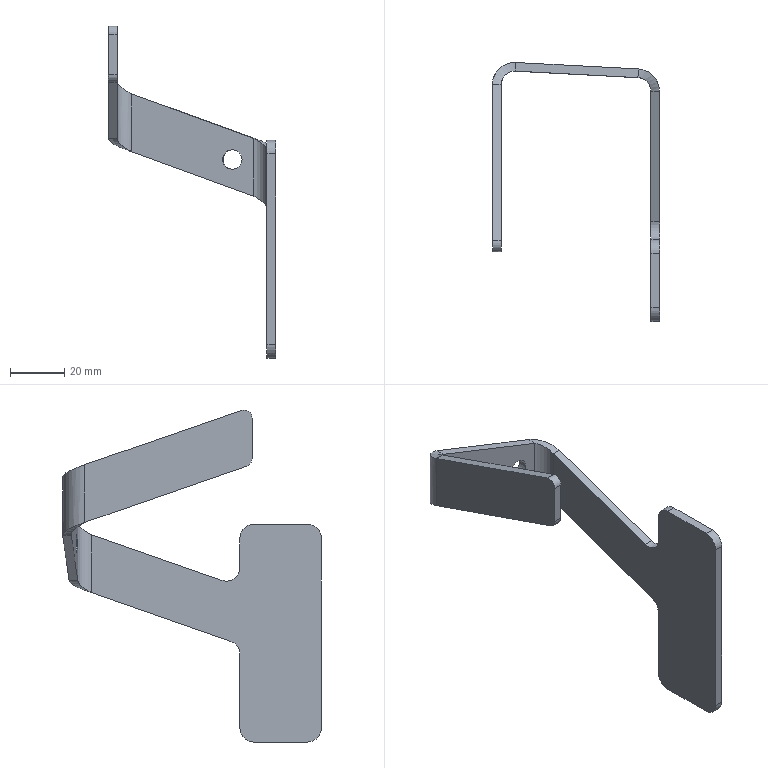Part | SolidWorks | features EdgeFlange 2, Fillet 2, ICE 2, FlatPattern 1, RefAxis 1, SMBaseFlange 1, SheetMetal 1 | 1 solid | 36 faces | box 61.639 x 95.405 x 122.483 mm | volume 19991 mm3 | plane 18 | cylinder 14 | spline 4 | commonest cylinder face diameters 10 x8 6 x2 7.2 x2 16.4 x2
STEP:
#1=CARTESIAN_POINT('',(3.429,-3.382,0.));
#2=VERTEX_POINT('',#1);
#3=CARTESIAN_POINT('',(-3.761,-3.009,0.));
#4=VERTEX_POINT('',#3);
#5=CARTESIAN_POINT('',(-0.166,-3.196,0.));
#6=DIRECTION('',(0.05188,0.9987,0.));
#7=DIRECTION('',(-0.9987,0.05188,0.));
#8=AXIS2_PLACEMENT_3D('',#5,#6,#7);
#9=CIRCLE('',#8,3.6);
#10=EDGE_CURVE('',#2,#4,#9,.T.);
#11=ORIENTED_EDGE('',*,*,#10,.F.);
#12=CARTESIAN_POINT('',(3.595,-0.1868,0.));
#13=VERTEX_POINT('',#12);
#14=CARTESIAN_POINT('',(3.076,-10.173,0.));
#15=DIRECTION('',(0.05188,0.9987,0.));
#16=VECTOR('',#15,1000.);
#17=LINE('',#14,#16);
#18=EDGE_CURVE('',#2,#13,#17,.T.);
#19=ORIENTED_EDGE('',*,*,#18,.T.);
#20=CARTESIAN_POINT('',(-3.595,0.1868,0.));
#21=VERTEX_POINT('',#20);
#22=CARTESIAN_POINT('',(0.,0.,0.));
#23=DIRECTION('',(0.05188,0.9987,0.));
#24=DIRECTION('',(-0.9987,0.05188,0.));
#25=AXIS2_PLACEMENT_3D('',#22,#23,#24);
#26=CIRCLE('',#25,3.6);
#27=EDGE_CURVE('',#13,#21,#26,.T.);
#28=ORIENTED_EDGE('',*,*,#27,.T.);
#29=CARTESIAN_POINT('',(-4.114,-9.8,0.));
#30=DIRECTION('',(0.05188,0.9987,0.));
#31=VECTOR('',#30,1000.);
#32=LINE('',#29,#31);
#33=EDGE_CURVE('',#4,#21,#32,.T.);
#34=ORIENTED_EDGE('',*,*,#33,.F.);
#35=EDGE_LOOP('',(#11,#19,#28,#34));
#36=FACE_OUTER_BOUND('',#35,.T.);
#37=CARTESIAN_POINT('',(-0.5188,-9.987,0.));
#38=DIRECTION('',(0.05188,0.9987,0.));
#39=DIRECTION('',(-0.9987,0.05188,0.));
#40=AXIS2_PLACEMENT_3D('',#37,#38,#39);
#41=CYLINDRICAL_SURFACE('',#40,3.6);
#42=ADVANCED_FACE('',(#36),#41,.F.);
#43=CARTESIAN_POINT('',(-0.166,-3.196,0.));
#44=DIRECTION('',(0.05188,0.9987,0.));
#45=DIRECTION('',(-0.9987,0.05188,0.));
#46=AXIS2_PLACEMENT_3D('',#43,#44,#45);
#47=CIRCLE('',#46,3.6);
#48=EDGE_CURVE('',#4,#2,#47,.T.);
#49=ORIENTED_EDGE('',*,*,#48,.T.);
#50=ORIENTED_EDGE('',*,*,#10,.T.);
#51=EDGE_LOOP('',(#49,#50));
#52=FACE_BOUND('',#51,.T.);
#53=CARTESIAN_POINT('',(7.795,-3.609,7.804));
#54=VERTEX_POINT('',#53);
#55=CARTESIAN_POINT('',(7.795,-3.609,-13.54));
#56=VERTEX_POINT('',#55);
#57=CARTESIAN_POINT('',(7.795,-3.609,7.804));
#58=DIRECTION('',(0.,0.,-1.));
#59=VECTOR('',#58,1000.);
#60=LINE('',#57,#59);
#61=EDGE_CURVE('',#54,#56,#60,.T.);
#62=ORIENTED_EDGE('',*,*,#61,.F.);
#63=CARTESIAN_POINT('',(-37.404,-1.261,24.256));
#64=VERTEX_POINT('',#63);
#65=CARTESIAN_POINT('',(-53.293,-0.4358,30.039));
#66=DIRECTION('',(-0.9386,0.04876,0.3416));
#67=VECTOR('',#66,1000.);
#68=LINE('',#65,#67);
#69=EDGE_CURVE('',#54,#64,#68,.T.);
#70=ORIENTED_EDGE('',*,*,#69,.T.);
#71=CARTESIAN_POINT('',(-37.404,-1.261,2.912));
#72=VERTEX_POINT('',#71);
#73=CARTESIAN_POINT('',(-37.404,-1.261,2.912));
#74=DIRECTION('',(0.,0.,1.));
#75=VECTOR('',#74,1000.);
#76=LINE('',#73,#75);
#77=EDGE_CURVE('',#72,#64,#76,.T.);
#78=ORIENTED_EDGE('',*,*,#77,.F.);
#79=CARTESIAN_POINT('',(-60.137,-0.08033,11.186));
#80=DIRECTION('',(0.9386,-0.04876,-0.3416));
#81=VECTOR('',#80,1000.);
#82=LINE('',#79,#81);
#83=EDGE_CURVE('',#72,#56,#82,.T.);
#84=ORIENTED_EDGE('',*,*,#83,.T.);
#85=EDGE_LOOP('',(#62,#70,#78,#84));
#86=FACE_OUTER_BOUND('',#85,.T.);
#87=CARTESIAN_POINT('',(-45.866,-0.8217,50.5));
#88=DIRECTION('',(0.05188,0.9987,0.));
#89=DIRECTION('',(-0.9987,0.05188,0.));
#90=AXIS2_PLACEMENT_3D('',#87,#88,#89);
#91=PLANE('',#90);
#92=ADVANCED_FACE('',(#52,#86),#91,.F.);
#93=CARTESIAN_POINT('',(0.,0.,0.));
#94=DIRECTION('',(0.05188,0.9987,0.));
#95=DIRECTION('',(-0.9987,0.05188,0.));
#96=AXIS2_PLACEMENT_3D('',#93,#94,#95);
#97=CIRCLE('',#96,3.6);
#98=EDGE_CURVE('',#21,#13,#97,.T.);
#99=ORIENTED_EDGE('',*,*,#98,.F.);
#100=ORIENTED_EDGE('',*,*,#27,.F.);
#101=EDGE_LOOP('',(#99,#100));
#102=FACE_BOUND('',#101,.T.);
#103=CARTESIAN_POINT('',(7.961,-0.4136,7.804));
#104=VERTEX_POINT('',#103);
#105=CARTESIAN_POINT('',(-37.238,1.934,24.256));
#106=VERTEX_POINT('',#105);
#107=CARTESIAN_POINT('',(-53.127,2.76,30.039));
#108=DIRECTION('',(-0.9386,0.04876,0.3416));
#109=VECTOR('',#108,1000.);
#110=LINE('',#107,#109);
#111=EDGE_CURVE('',#104,#106,#110,.T.);
#112=ORIENTED_EDGE('',*,*,#111,.F.);
#113=CARTESIAN_POINT('',(7.961,-0.4136,-13.54));
#114=VERTEX_POINT('',#113);
#115=CARTESIAN_POINT('',(7.961,-0.4136,7.804));
#116=DIRECTION('',(0.,0.,-1.));
#117=VECTOR('',#116,1000.);
#118=LINE('',#115,#117);
#119=EDGE_CURVE('',#104,#114,#118,.T.);
#120=ORIENTED_EDGE('',*,*,#119,.T.);
#121=CARTESIAN_POINT('',(-37.238,1.934,2.912));
#122=VERTEX_POINT('',#121);
#123=CARTESIAN_POINT('',(-59.971,3.115,11.186));
#124=DIRECTION('',(0.9386,-0.04876,-0.3416));
#125=VECTOR('',#124,1000.);
#126=LINE('',#123,#125);
#127=EDGE_CURVE('',#122,#114,#126,.T.);
#128=ORIENTED_EDGE('',*,*,#127,.F.);
#129=CARTESIAN_POINT('',(-37.238,1.934,2.912));
#130=DIRECTION('',(0.,0.,1.));
#131=VECTOR('',#130,1000.);
#132=LINE('',#129,#131);
#133=EDGE_CURVE('',#122,#106,#132,.T.);
#134=ORIENTED_EDGE('',*,*,#133,.T.);
#135=EDGE_LOOP('',(#112,#120,#128,#134));
#136=FACE_OUTER_BOUND('',#135,.T.);
#137=CARTESIAN_POINT('',(-45.7,2.374,50.5));
#138=DIRECTION('',(0.05188,0.9987,0.));
#139=DIRECTION('',(-0.9987,0.05188,0.));
#140=AXIS2_PLACEMENT_3D('',#137,#138,#139);
#141=PLANE('',#140);
#142=ADVANCED_FACE('',(#102,#136),#141,.T.);
#143=CARTESIAN_POINT('',(7.795,-3.609,7.804));
#144=DIRECTION('',(0.05188,0.9987,0.));
#145=VECTOR('',#144,1000.);
#146=LINE('',#143,#145);
#147=EDGE_CURVE('',#54,#104,#146,.T.);
#148=ORIENTED_EDGE('',*,*,#147,.T.);
#149=ORIENTED_EDGE('',*,*,#111,.T.);
#150=CARTESIAN_POINT('',(-37.404,-1.261,24.256));
#151=DIRECTION('',(0.05188,0.9987,0.));
#152=VECTOR('',#151,1000.);
#153=LINE('',#150,#152);
#154=EDGE_CURVE('',#64,#106,#153,.T.);
#155=ORIENTED_EDGE('',*,*,#154,.F.);
#156=ORIENTED_EDGE('',*,*,#69,.F.);
#157=EDGE_LOOP('',(#148,#149,#155,#156));
#158=FACE_OUTER_BOUND('',#157,.T.);
#159=CARTESIAN_POINT('',(-53.127,2.76,30.039));
#160=DIRECTION('',(0.3412,-0.01772,0.9398));
#161=DIRECTION('',(-0.9386,0.04876,0.3416));
#162=AXIS2_PLACEMENT_3D('',#159,#160,#161);
#163=PLANE('',#162);
#164=ADVANCED_FACE('',(#158),#163,.T.);
#165=CARTESIAN_POINT('',(7.795,-3.609,-13.54));
#166=DIRECTION('',(0.05188,0.9987,0.));
#167=VECTOR('',#166,1000.);
#168=LINE('',#165,#167);
#169=EDGE_CURVE('',#56,#114,#168,.T.);
#170=ORIENTED_EDGE('',*,*,#169,.F.);
#171=ORIENTED_EDGE('',*,*,#83,.F.);
#172=CARTESIAN_POINT('',(-37.404,-1.261,2.912));
#173=DIRECTION('',(0.05188,0.9987,0.));
#174=VECTOR('',#173,1000.);
#175=LINE('',#172,#174);
#176=EDGE_CURVE('',#72,#122,#175,.T.);
#177=ORIENTED_EDGE('',*,*,#176,.T.);
#178=ORIENTED_EDGE('',*,*,#127,.T.);
#179=EDGE_LOOP('',(#170,#171,#177,#178));
#180=FACE_OUTER_BOUND('',#179,.T.);
#181=CARTESIAN_POINT('',(-59.971,3.115,11.186));
#182=DIRECTION('',(-0.3412,0.01772,-0.9398));
#183=DIRECTION('',(0.9386,-0.04876,-0.3416));
#184=AXIS2_PLACEMENT_3D('',#181,#182,#183);
#185=PLANE('',#184);
#186=ADVANCED_FACE('',(#180),#185,.T.);
#187=CARTESIAN_POINT('',(-42.664,-6.257,29.104));
#188=VERTEX_POINT('',#187);
#189=CARTESIAN_POINT('',(-45.864,-6.258,29.104));
#190=VERTEX_POINT('',#189);
#191=CARTESIAN_POINT('',(-45.864,-6.258,29.104));
#192=DIRECTION('',(-1.,-0.0004585,0.));
#193=VECTOR('',#192,1000.);
#194=LINE('',#191,#193);
#195=EDGE_CURVE('',#188,#190,#194,.T.);
#196=ORIENTED_EDGE('',*,*,#195,.F.);
#197=CARTESIAN_POINT('',(-37.404,-1.261,24.256));
#198=CARTESIAN_POINT('',(-37.745,-1.244,24.46));
#199=CARTESIAN_POINT('',(-38.083,-1.261,24.661));
#200=CARTESIAN_POINT('',(-38.748,-1.362,25.062));
#201=CARTESIAN_POINT('',(-39.077,-1.446,25.264));
#202=CARTESIAN_POINT('',(-39.716,-1.682,25.671));
#203=CARTESIAN_POINT('',(-40.019,-1.831,25.872));
#204=CARTESIAN_POINT('',(-40.59,-2.187,26.274));
#205=CARTESIAN_POINT('',(-40.86,-2.395,26.476));
#206=CARTESIAN_POINT('',(-41.353,-2.863,26.883));
#207=CARTESIAN_POINT('',(-41.573,-3.12,27.083));
#208=CARTESIAN_POINT('',(-41.862,-3.534,27.385));
#209=CARTESIAN_POINT('',(-41.951,-3.677,27.486));
#210=CARTESIAN_POINT('',(-42.116,-3.973,27.688));
#211=CARTESIAN_POINT('',(-42.191,-4.126,27.79));
#212=CARTESIAN_POINT('',(-42.392,-4.595,28.094));
#213=CARTESIAN_POINT('',(-42.493,-4.917,28.295));
#214=CARTESIAN_POINT('',(-42.629,-5.576,28.697));
#215=CARTESIAN_POINT('',(-42.664,-5.916,28.9));
#216=CARTESIAN_POINT('',(-42.664,-6.257,29.104));
#217=B_SPLINE_CURVE_WITH_KNOTS('',3,(#197,#198,#199,#200,#201,#202,#203,#204,#205,#206,#207,#208,#209,#210,#211,#212,#213,#214,#215,#216),.UNSPECIFIED.,.F.,.F.,(4,2,2,2,2,2,2,2,2,4),(0.,0.001176,0.002352,0.003527,0.004703,0.005879,0.006467,0.007055,0.00823,0.009406),.UNSPECIFIED.);
#218=EDGE_CURVE('',#64,#188,#217,.T.);
#219=ORIENTED_EDGE('',*,*,#218,.F.);
#220=ORIENTED_EDGE('',*,*,#154,.T.);
#221=CARTESIAN_POINT('',(-37.238,1.934,24.256));
#222=CARTESIAN_POINT('',(-37.797,1.963,24.46));
#223=CARTESIAN_POINT('',(-38.349,1.935,24.66));
#224=CARTESIAN_POINT('',(-39.167,1.811,24.961));
#225=CARTESIAN_POINT('',(-39.438,1.756,25.062));
#226=CARTESIAN_POINT('',(-39.976,1.618,25.264));
#227=CARTESIAN_POINT('',(-40.244,1.534,25.366));
#228=CARTESIAN_POINT('',(-41.026,1.245,25.67));
#229=CARTESIAN_POINT('',(-41.522,1.002,25.87));
#230=CARTESIAN_POINT('',(-42.461,0.4186,26.273));
#231=CARTESIAN_POINT('',(-42.907,0.07379,26.477));
#232=CARTESIAN_POINT('',(-43.71,-0.6881,26.88));
#233=CARTESIAN_POINT('',(-44.07,-1.106,27.08));
#234=CARTESIAN_POINT('',(-44.546,-1.789,27.383));
#235=CARTESIAN_POINT('',(-44.695,-2.027,27.485));
#236=CARTESIAN_POINT('',(-44.966,-2.513,27.688));
#237=CARTESIAN_POINT('',(-45.088,-2.762,27.789));
#238=CARTESIAN_POINT('',(-45.415,-3.522,28.09));
#239=CARTESIAN_POINT('',(-45.581,-4.049,28.291));
#240=CARTESIAN_POINT('',(-45.807,-5.142,28.697));
#241=CARTESIAN_POINT('',(-45.864,-5.699,28.9));
#242=CARTESIAN_POINT('',(-45.864,-6.258,29.104));
#243=B_SPLINE_CURVE_WITH_KNOTS('',3,(#221,#222,#223,#224,#225,#226,#227,#228,#229,#230,#231,#232,#233,#234,#235,#236,#237,#238,#239,#240,#241,#242),.UNSPECIFIED.,.F.,.F.,(4,2,2,2,2,2,2,2,2,2,4),(0.,0.001761,0.002641,0.003522,0.005283,0.007043,0.008804,0.009685,0.01057,0.01233,0.01409),.UNSPECIFIED.);
#244=EDGE_CURVE('',#106,#190,#243,.T.);
#245=ORIENTED_EDGE('',*,*,#244,.T.);
#246=EDGE_LOOP('',(#196,#219,#220,#245));
#247=FACE_OUTER_BOUND('',#246,.T.);
#248=CARTESIAN_POINT('',(-37.236,1.966,24.256));
#249=CARTESIAN_POINT('',(-38.349,2.024,24.66));
#250=CARTESIAN_POINT('',(-39.472,1.853,25.064));
#251=CARTESIAN_POINT('',(-41.561,1.081,25.872));
#252=CARTESIAN_POINT('',(-42.525,0.481,26.276));
#253=CARTESIAN_POINT('',(-44.14,-1.053,27.084));
#254=CARTESIAN_POINT('',(-44.789,-1.985,27.488));
#255=CARTESIAN_POINT('',(-45.668,-4.032,28.296));
#256=CARTESIAN_POINT('',(-45.896,-5.145,28.7));
#257=CARTESIAN_POINT('',(-45.896,-6.258,29.104));
#258=CARTESIAN_POINT('',(-37.238,1.934,24.256));
#259=CARTESIAN_POINT('',(-38.346,1.992,24.66));
#260=CARTESIAN_POINT('',(-39.465,1.822,25.064));
#261=CARTESIAN_POINT('',(-41.546,1.053,25.872));
#262=CARTESIAN_POINT('',(-42.507,0.4548,26.276));
#263=CARTESIAN_POINT('',(-44.115,-1.073,27.084));
#264=CARTESIAN_POINT('',(-44.762,-2.002,27.488));
#265=CARTESIAN_POINT('',(-45.636,-4.04,28.296));
#266=CARTESIAN_POINT('',(-45.864,-5.149,28.7));
#267=CARTESIAN_POINT('',(-45.864,-6.258,29.104));
#268=CARTESIAN_POINT('',(-37.404,-1.261,24.256));
#269=CARTESIAN_POINT('',(-38.08,-1.226,24.66));
#270=CARTESIAN_POINT('',(-38.762,-1.33,25.064));
#271=CARTESIAN_POINT('',(-40.031,-1.799,25.872));
#272=CARTESIAN_POINT('',(-40.617,-2.163,26.276));
#273=CARTESIAN_POINT('',(-41.597,-3.095,27.084));
#274=CARTESIAN_POINT('',(-41.992,-3.661,27.488));
#275=CARTESIAN_POINT('',(-42.525,-4.904,28.296));
#276=CARTESIAN_POINT('',(-42.664,-5.58,28.7));
#277=CARTESIAN_POINT('',(-42.664,-6.257,29.104));
#278=CARTESIAN_POINT('',(-37.406,-1.294,24.256));
#279=CARTESIAN_POINT('',(-38.077,-1.259,24.66));
#280=CARTESIAN_POINT('',(-38.755,-1.362,25.064));
#281=CARTESIAN_POINT('',(-40.015,-1.828,25.872));
#282=CARTESIAN_POINT('',(-40.597,-2.19,26.276));
#283=CARTESIAN_POINT('',(-41.572,-3.115,27.084));
#284=CARTESIAN_POINT('',(-41.964,-3.678,27.488));
#285=CARTESIAN_POINT('',(-42.494,-4.913,28.296));
#286=CARTESIAN_POINT('',(-42.632,-5.585,28.7));
#287=CARTESIAN_POINT('',(-42.631,-6.257,29.104));
#288=B_SPLINE_SURFACE_WITH_KNOTS('',1,3,((#248,#249,#250,#251,#252,#253,#254,#255,#256,#257),(#258,#259,#260,#261,#262,#263,#264,#265,#266,#267),(#268,#269,#270,#271,#272,#273,#274,#275,#276,#277),(#278,#279,#280,#281,#282,#283,#284,#285,#286,#287)),.UNSPECIFIED.,.F.,.F.,.F.,(2,1,1,2),(4,2,2,2,4),(-0.01,0.,1.,1.01),(0.,0.25,0.5,0.75,1.),.UNSPECIFIED.);
#289=ADVANCED_FACE('',(#247),#288,.F.);
#290=CARTESIAN_POINT('',(-42.664,-6.257,7.82));
#291=VERTEX_POINT('',#290);
#292=CARTESIAN_POINT('',(-42.664,-6.257,7.82));
#293=CARTESIAN_POINT('',(-42.664,-5.915,7.613));
#294=CARTESIAN_POINT('',(-42.629,-5.579,7.41));
#295=CARTESIAN_POINT('',(-42.494,-4.919,7.003));
#296=CARTESIAN_POINT('',(-42.392,-4.595,6.798));
#297=CARTESIAN_POINT('',(-42.123,-3.968,6.386));
#298=CARTESIAN_POINT('',(-41.959,-3.673,6.182));
#299=CARTESIAN_POINT('',(-41.573,-3.12,5.775));
#300=CARTESIAN_POINT('',(-41.352,-2.861,5.57));
#301=CARTESIAN_POINT('',(-40.857,-2.393,5.158));
#302=CARTESIAN_POINT('',(-40.59,-2.186,4.955));
#303=CARTESIAN_POINT('',(-40.161,-1.919,4.649));
#304=CARTESIAN_POINT('',(-40.013,-1.838,4.547));
#305=CARTESIAN_POINT('',(-39.709,-1.689,4.342));
#306=CARTESIAN_POINT('',(-39.551,-1.621,4.239));
#307=CARTESIAN_POINT('',(-38.754,-1.328,3.725));
#308=CARTESIAN_POINT('',(-38.086,-1.226,3.325));
#309=CARTESIAN_POINT('',(-37.404,-1.261,2.912));
#310=B_SPLINE_CURVE_WITH_KNOTS('',3,(#292,#293,#294,#295,#296,#297,#298,#299,#300,#301,#302,#303,#304,#305,#306,#307,#308,#309),.UNSPECIFIED.,.F.,.F.,(4,2,2,2,2,2,2,2,4),(0.,0.001181,0.002361,0.003542,0.004723,0.005903,0.006494,0.007084,0.009446),.UNSPECIFIED.);
#311=EDGE_CURVE('',#291,#72,#310,.T.);
#312=ORIENTED_EDGE('',*,*,#311,.F.);
#313=CARTESIAN_POINT('',(-45.864,-6.258,7.82));
#314=VERTEX_POINT('',#313);
#315=CARTESIAN_POINT('',(-42.664,-6.257,7.82));
#316=DIRECTION('',(-1.,-0.0004585,0.));
#317=VECTOR('',#316,1000.);
#318=LINE('',#315,#317);
#319=EDGE_CURVE('',#291,#314,#318,.T.);
#320=ORIENTED_EDGE('',*,*,#319,.T.);
#321=CARTESIAN_POINT('',(-45.864,-6.258,7.82));
#322=CARTESIAN_POINT('',(-45.864,-5.699,7.614));
#323=CARTESIAN_POINT('',(-45.807,-5.148,7.411));
#324=CARTESIAN_POINT('',(-45.641,-4.338,7.106));
#325=CARTESIAN_POINT('',(-45.572,-4.07,7.004));
#326=CARTESIAN_POINT('',(-45.406,-3.54,6.799));
#327=CARTESIAN_POINT('',(-45.309,-3.277,6.696));
#328=CARTESIAN_POINT('',(-44.98,-2.511,6.388));
#329=CARTESIAN_POINT('',(-44.712,-2.028,6.186));
#330=CARTESIAN_POINT('',(-44.081,-1.12,5.778));
#331=CARTESIAN_POINT('',(-43.714,-0.6921,5.571));
#332=CARTESIAN_POINT('',(-42.912,0.07036,5.163));
#333=CARTESIAN_POINT('',(-42.475,0.4084,4.96));
#334=CARTESIAN_POINT('',(-41.769,0.8489,4.654));
#335=CARTESIAN_POINT('',(-41.524,0.9852,4.55));
#336=CARTESIAN_POINT('',(-41.024,1.23,4.345));
#337=CARTESIAN_POINT('',(-40.77,1.339,4.243));
#338=CARTESIAN_POINT('',(-39.994,1.627,3.938));
#339=CARTESIAN_POINT('',(-39.459,1.766,3.735));
#340=CARTESIAN_POINT('',(-38.356,1.935,3.324));
#341=CARTESIAN_POINT('',(-37.797,1.963,3.118));
#342=CARTESIAN_POINT('',(-37.238,1.934,2.912));
#343=B_SPLINE_CURVE_WITH_KNOTS('',3,(#321,#322,#323,#324,#325,#326,#327,#328,#329,#330,#331,#332,#333,#334,#335,#336,#337,#338,#339,#340,#341,#342),.UNSPECIFIED.,.F.,.F.,(4,2,2,2,2,2,2,2,2,2,4),(0.,0.001763,0.002645,0.003527,0.00529,0.007054,0.008817,0.009699,0.01058,0.01234,0.01411),.UNSPECIFIED.);
#344=EDGE_CURVE('',#314,#122,#343,.T.);
#345=ORIENTED_EDGE('',*,*,#344,.T.);
#346=ORIENTED_EDGE('',*,*,#176,.F.);
#347=EDGE_LOOP('',(#312,#320,#345,#346));
#348=FACE_OUTER_BOUND('',#347,.T.);
#349=CARTESIAN_POINT('',(-45.896,-6.258,7.82));
#350=CARTESIAN_POINT('',(-45.896,-5.145,7.411));
#351=CARTESIAN_POINT('',(-45.668,-4.032,7.002));
#352=CARTESIAN_POINT('',(-44.789,-1.985,6.184));
#353=CARTESIAN_POINT('',(-44.14,-1.053,5.775));
#354=CARTESIAN_POINT('',(-42.525,0.481,4.957));
#355=CARTESIAN_POINT('',(-41.561,1.081,4.548));
#356=CARTESIAN_POINT('',(-39.472,1.853,3.73));
#357=CARTESIAN_POINT('',(-38.349,2.024,3.321));
#358=CARTESIAN_POINT('',(-37.236,1.966,2.912));
#359=CARTESIAN_POINT('',(-45.864,-6.258,7.82));
#360=CARTESIAN_POINT('',(-45.864,-5.149,7.411));
#361=CARTESIAN_POINT('',(-45.636,-4.04,7.002));
#362=CARTESIAN_POINT('',(-44.762,-2.002,6.184));
#363=CARTESIAN_POINT('',(-44.115,-1.073,5.775));
#364=CARTESIAN_POINT('',(-42.507,0.4548,4.957));
#365=CARTESIAN_POINT('',(-41.546,1.053,4.548));
#366=CARTESIAN_POINT('',(-39.465,1.822,3.73));
#367=CARTESIAN_POINT('',(-38.346,1.992,3.321));
#368=CARTESIAN_POINT('',(-37.238,1.934,2.912));
#369=CARTESIAN_POINT('',(-42.664,-6.257,7.82));
#370=CARTESIAN_POINT('',(-42.664,-5.58,7.411));
#371=CARTESIAN_POINT('',(-42.525,-4.904,7.002));
#372=CARTESIAN_POINT('',(-41.992,-3.661,6.184));
#373=CARTESIAN_POINT('',(-41.597,-3.095,5.775));
#374=CARTESIAN_POINT('',(-40.617,-2.163,4.957));
#375=CARTESIAN_POINT('',(-40.031,-1.799,4.548));
#376=CARTESIAN_POINT('',(-38.762,-1.33,3.73));
#377=CARTESIAN_POINT('',(-38.08,-1.226,3.321));
#378=CARTESIAN_POINT('',(-37.404,-1.261,2.912));
#379=CARTESIAN_POINT('',(-42.631,-6.257,7.82));
#380=CARTESIAN_POINT('',(-42.632,-5.585,7.411));
#381=CARTESIAN_POINT('',(-42.494,-4.913,7.002));
#382=CARTESIAN_POINT('',(-41.964,-3.678,6.184));
#383=CARTESIAN_POINT('',(-41.572,-3.115,5.775));
#384=CARTESIAN_POINT('',(-40.597,-2.19,4.957));
#385=CARTESIAN_POINT('',(-40.015,-1.828,4.548));
#386=CARTESIAN_POINT('',(-38.755,-1.362,3.73));
#387=CARTESIAN_POINT('',(-38.077,-1.259,3.321));
#388=CARTESIAN_POINT('',(-37.406,-1.294,2.912));
#389=B_SPLINE_SURFACE_WITH_KNOTS('',1,3,((#349,#350,#351,#352,#353,#354,#355,#356,#357,#358),(#359,#360,#361,#362,#363,#364,#365,#366,#367,#368),(#369,#370,#371,#372,#373,#374,#375,#376,#377,#378),(#379,#380,#381,#382,#383,#384,#385,#386,#387,#388)),.UNSPECIFIED.,.F.,.F.,.F.,(2,1,1,2),(4,2,2,2,4),(-0.01,0.,1.,1.01),(0.,0.25,0.5,0.75,1.),.UNSPECIFIED.);
#390=ADVANCED_FACE('',(#348),#389,.F.);
#391=ORIENTED_EDGE('',*,*,#133,.F.);
#392=ORIENTED_EDGE('',*,*,#344,.F.);
#393=CARTESIAN_POINT('',(-45.864,-6.258,29.104));
#394=DIRECTION('',(0.,0.,1.));
#395=VECTOR('',#394,1000.);
#396=LINE('',#393,#395);
#397=EDGE_CURVE('',#314,#190,#396,.T.);
#398=ORIENTED_EDGE('',*,*,#397,.T.);
#399=ORIENTED_EDGE('',*,*,#244,.F.);
#400=EDGE_LOOP('',(#391,#392,#398,#399));
#401=FACE_OUTER_BOUND('',#400,.T.);
#402=CARTESIAN_POINT('',(-37.664,-6.255,2.912));
#403=DIRECTION('',(0.,0.,-1.));
#404=DIRECTION('',(-1.,-0.0004585,0.));
#405=AXIS2_PLACEMENT_3D('',#402,#403,#404);
#406=CYLINDRICAL_SURFACE('',#405,8.2);
#407=ADVANCED_FACE('',(#401),#406,.T.);
#408=ORIENTED_EDGE('',*,*,#77,.T.);
#409=ORIENTED_EDGE('',*,*,#218,.T.);
#410=CARTESIAN_POINT('',(-42.664,-6.257,29.104));
#411=DIRECTION('',(0.,0.,-1.));
#412=VECTOR('',#411,1000.);
#413=LINE('',#410,#412);
#414=EDGE_CURVE('',#188,#291,#413,.T.);
#415=ORIENTED_EDGE('',*,*,#414,.T.);
#416=ORIENTED_EDGE('',*,*,#311,.T.);
#417=EDGE_LOOP('',(#408,#409,#415,#416));
#418=FACE_OUTER_BOUND('',#417,.T.);
#419=CARTESIAN_POINT('',(-37.664,-6.255,2.912));
#420=DIRECTION('',(0.,0.,-1.));
#421=DIRECTION('',(-1.,-0.0004585,0.));
#422=AXIS2_PLACEMENT_3D('',#419,#420,#421);
#423=CYLINDRICAL_SURFACE('',#422,5.);
#424=ADVANCED_FACE('',(#418),#423,.F.);
#425=CARTESIAN_POINT('',(-42.636,-65.899,28.517));
#426=VERTEX_POINT('',#425);
#427=CARTESIAN_POINT('',(-42.635,-67.916,29.216));
#428=DIRECTION('',(0.0004331,-0.9447,0.3278));
#429=VECTOR('',#428,1000.);
#430=LINE('',#427,#429);
#431=EDGE_CURVE('',#291,#426,#430,.T.);
#432=ORIENTED_EDGE('',*,*,#431,.T.);
#433=CARTESIAN_POINT('',(-45.836,-65.901,28.517));
#434=VERTEX_POINT('',#433);
#435=CARTESIAN_POINT('',(-45.836,-65.901,28.517));
#436=DIRECTION('',(-1.,-0.0004585,0.));
#437=VECTOR('',#436,1000.);
#438=LINE('',#435,#437);
#439=EDGE_CURVE('',#426,#434,#438,.T.);
#440=ORIENTED_EDGE('',*,*,#439,.T.);
#441=CARTESIAN_POINT('',(-45.867,1.581,5.1));
#442=DIRECTION('',(0.0004331,-0.9447,0.3278));
#443=VECTOR('',#442,1000.);
#444=LINE('',#441,#443);
#445=EDGE_CURVE('',#314,#434,#444,.T.);
#446=ORIENTED_EDGE('',*,*,#445,.F.);
#447=ORIENTED_EDGE('',*,*,#319,.F.);
#448=EDGE_LOOP('',(#432,#440,#446,#447));
#449=FACE_OUTER_BOUND('',#448,.T.);
#450=CARTESIAN_POINT('',(-45.835,-67.917,29.216));
#451=DIRECTION('',(-0.0001503,0.3278,0.9447));
#452=DIRECTION('',(0.,-0.9447,0.3278));
#453=AXIS2_PLACEMENT_3D('',#450,#451,#452);
#454=PLANE('',#453);
#455=ADVANCED_FACE('',(#449),#454,.F.);
#456=CARTESIAN_POINT('',(-45.837,-63.934,49.118));
#457=VERTEX_POINT('',#456);
#458=CARTESIAN_POINT('',(-45.87,8.173,24.096));
#459=DIRECTION('',(-0.0004331,0.9447,-0.3278));
#460=VECTOR('',#459,1000.);
#461=LINE('',#458,#460);
#462=EDGE_CURVE('',#457,#190,#461,.T.);
#463=ORIENTED_EDGE('',*,*,#462,.F.);
#464=CARTESIAN_POINT('',(-42.637,-63.932,49.118));
#465=VERTEX_POINT('',#464);
#466=CARTESIAN_POINT('',(-45.837,-63.934,49.118));
#467=DIRECTION('',(1.,0.0004585,0.));
#468=VECTOR('',#467,1000.);
#469=LINE('',#466,#468);
#470=EDGE_CURVE('',#457,#465,#469,.T.);
#471=ORIENTED_EDGE('',*,*,#470,.T.);
#472=CARTESIAN_POINT('',(-42.666,-0.9879,27.275));
#473=DIRECTION('',(-0.0004331,0.9447,-0.3278));
#474=VECTOR('',#473,1000.);
#475=LINE('',#472,#474);
#476=EDGE_CURVE('',#465,#188,#475,.T.);
#477=ORIENTED_EDGE('',*,*,#476,.T.);
#478=ORIENTED_EDGE('',*,*,#195,.T.);
#479=EDGE_LOOP('',(#463,#471,#477,#478));
#480=FACE_OUTER_BOUND('',#479,.T.);
#481=CARTESIAN_POINT('',(-45.866,-0.9894,27.275));
#482=DIRECTION('',(0.0001503,-0.3278,-0.9447));
#483=DIRECTION('',(0.,0.9447,-0.3278));
#484=AXIS2_PLACEMENT_3D('',#481,#482,#483);
#485=PLANE('',#484);
#486=ADVANCED_FACE('',(#480),#485,.F.);
#487=CARTESIAN_POINT('',(-45.835,-67.917,31.351));
#488=VERTEX_POINT('',#487);
#489=CARTESIAN_POINT('',(-45.835,-67.917,46.283));
#490=VERTEX_POINT('',#489);
#491=CARTESIAN_POINT('',(-45.835,-67.917,0.));
#492=DIRECTION('',(0.,0.,1.));
#493=VECTOR('',#492,1000.);
#494=LINE('',#491,#493);
#495=EDGE_CURVE('',#488,#490,#494,.T.);
#496=ORIENTED_EDGE('',*,*,#495,.T.);
#497=CARTESIAN_POINT('',(-45.837,-64.917,46.283));
#498=DIRECTION('',(-1.,-0.0004585,0.));
#499=DIRECTION('',(-0.0004585,1.,0.));
#500=AXIS2_PLACEMENT_3D('',#497,#498,#499);
#501=CIRCLE('',#500,3.);
#502=EDGE_CURVE('',#490,#457,#501,.T.);
#503=ORIENTED_EDGE('',*,*,#502,.T.);
#504=ORIENTED_EDGE('',*,*,#462,.T.);
#505=ORIENTED_EDGE('',*,*,#397,.F.);
#506=ORIENTED_EDGE('',*,*,#445,.T.);
#507=CARTESIAN_POINT('',(-45.837,-64.917,31.351));
#508=DIRECTION('',(-1.,-0.0004585,0.));
#509=DIRECTION('',(-0.0004585,1.,0.));
#510=AXIS2_PLACEMENT_3D('',#507,#508,#509);
#511=CIRCLE('',#510,3.);
#512=EDGE_CURVE('',#434,#488,#511,.T.);
#513=ORIENTED_EDGE('',*,*,#512,.T.);
#514=EDGE_LOOP('',(#496,#503,#504,#505,#506,#513));
#515=FACE_OUTER_BOUND('',#514,.T.);
#516=CARTESIAN_POINT('',(-45.866,-0.1887,0.));
#517=DIRECTION('',(1.,0.0004585,0.));
#518=DIRECTION('',(-0.0004585,1.,0.));
#519=AXIS2_PLACEMENT_3D('',#516,#517,#518);
#520=PLANE('',#519);
#521=ADVANCED_FACE('',(#515),#520,.F.);
#522=ORIENTED_EDGE('',*,*,#476,.F.);
#523=CARTESIAN_POINT('',(-42.635,-67.916,46.283));
#524=VERTEX_POINT('',#523);
#525=CARTESIAN_POINT('',(-42.637,-64.916,46.283));
#526=DIRECTION('',(1.,0.0004585,0.));
#527=DIRECTION('',(-0.0004585,1.,0.));
#528=AXIS2_PLACEMENT_3D('',#525,#526,#527);
#529=CIRCLE('',#528,3.);
#530=EDGE_CURVE('',#465,#524,#529,.T.);
#531=ORIENTED_EDGE('',*,*,#530,.T.);
#532=CARTESIAN_POINT('',(-42.635,-67.916,31.351));
#533=VERTEX_POINT('',#532);
#534=CARTESIAN_POINT('',(-42.635,-67.916,50.5));
#535=DIRECTION('',(0.,0.,1.));
#536=VECTOR('',#535,1000.);
#537=LINE('',#534,#536);
#538=EDGE_CURVE('',#533,#524,#537,.T.);
#539=ORIENTED_EDGE('',*,*,#538,.F.);
#540=CARTESIAN_POINT('',(-42.637,-64.916,31.351));
#541=DIRECTION('',(1.,0.0004585,0.));
#542=DIRECTION('',(-0.0004585,1.,0.));
#543=AXIS2_PLACEMENT_3D('',#540,#541,#542);
#544=CIRCLE('',#543,3.);
#545=EDGE_CURVE('',#533,#426,#544,.T.);
#546=ORIENTED_EDGE('',*,*,#545,.T.);
#547=ORIENTED_EDGE('',*,*,#431,.F.);
#548=ORIENTED_EDGE('',*,*,#414,.F.);
#549=EDGE_LOOP('',(#522,#531,#539,#546,#547,#548));
#550=FACE_OUTER_BOUND('',#549,.T.);
#551=CARTESIAN_POINT('',(-42.666,-0.1873,0.));
#552=DIRECTION('',(1.,0.0004585,0.));
#553=DIRECTION('',(-0.0004585,1.,0.));
#554=AXIS2_PLACEMENT_3D('',#551,#552,#553);
#555=PLANE('',#554);
#556=ADVANCED_FACE('',(#550),#555,.T.);
#557=ORIENTED_EDGE('',*,*,#538,.T.);
#558=CARTESIAN_POINT('',(-45.835,-67.917,46.283));
#559=DIRECTION('',(-1.,-0.0004585,0.));
#560=VECTOR('',#559,1000.);
#561=LINE('',#558,#560);
#562=EDGE_CURVE('',#524,#490,#561,.T.);
#563=ORIENTED_EDGE('',*,*,#562,.T.);
#564=ORIENTED_EDGE('',*,*,#495,.F.);
#565=CARTESIAN_POINT('',(-45.835,-67.917,31.351));
#566=DIRECTION('',(1.,0.0004585,0.));
#567=VECTOR('',#566,1000.);
#568=LINE('',#565,#567);
#569=EDGE_CURVE('',#488,#533,#568,.T.);
#570=ORIENTED_EDGE('',*,*,#569,.T.);
#571=EDGE_LOOP('',(#557,#563,#564,#570));
#572=FACE_OUTER_BOUND('',#571,.T.);
#573=CARTESIAN_POINT('',(-45.835,-67.917,50.5));
#574=DIRECTION('',(-0.0004585,1.,0.));
#575=DIRECTION('',(-1.,-0.0004585,0.));
#576=AXIS2_PLACEMENT_3D('',#573,#574,#575);
#577=PLANE('',#576);
#578=ADVANCED_FACE('',(#572),#577,.F.);
#579=CARTESIAN_POINT('',(12.536,-8.6,-18.086));
#580=VERTEX_POINT('',#579);
#581=CARTESIAN_POINT('',(15.736,-8.599,-18.086));
#582=VERTEX_POINT('',#581);
#583=CARTESIAN_POINT('',(15.736,-8.599,-18.086));
#584=DIRECTION('',(1.,0.0004585,0.));
#585=VECTOR('',#584,1000.);
#586=LINE('',#583,#585);
#587=EDGE_CURVE('',#580,#582,#586,.T.);
#588=ORIENTED_EDGE('',*,*,#587,.F.);
#589=CARTESIAN_POINT('',(7.795,-3.609,-13.54));
#590=CARTESIAN_POINT('',(8.433,-3.642,-13.922));
#591=CARTESIAN_POINT('',(9.047,-3.794,-14.294));
#592=CARTESIAN_POINT('',(9.915,-4.193,-14.866));
#593=CARTESIAN_POINT('',(10.19,-4.353,-15.055));
#594=CARTESIAN_POINT('',(10.702,-4.719,-15.432));
#595=CARTESIAN_POINT('',(10.94,-4.926,-15.62));
#596=CARTESIAN_POINT('',(11.378,-5.387,-16.001));
#597=CARTESIAN_POINT('',(11.575,-5.638,-16.191));
#598=CARTESIAN_POINT('',(11.915,-6.168,-16.568));
#599=CARTESIAN_POINT('',(12.06,-6.449,-16.756));
#600=CARTESIAN_POINT('',(12.296,-7.038,-17.137));
#601=CARTESIAN_POINT('',(12.386,-7.345,-17.328));
#602=CARTESIAN_POINT('',(12.505,-7.966,-17.706));
#603=CARTESIAN_POINT('',(12.536,-8.281,-17.895));
#604=CARTESIAN_POINT('',(12.536,-8.6,-18.086));
#605=B_SPLINE_CURVE_WITH_KNOTS('',3,(#589,#590,#591,#592,#593,#594,#595,#596,#597,#598,#599,#600,#601,#602,#603,#604),.UNSPECIFIED.,.F.,.F.,(4,2,2,2,2,2,2,4),(0.,0.002201,0.003301,0.004401,0.005502,0.006602,0.007702,0.008803),.UNSPECIFIED.);
#606=EDGE_CURVE('',#56,#580,#605,.T.);
#607=ORIENTED_EDGE('',*,*,#606,.F.);
#608=ORIENTED_EDGE('',*,*,#169,.T.);
#609=CARTESIAN_POINT('',(7.961,-0.4136,-13.54));
#610=CARTESIAN_POINT('',(8.484,-0.4407,-13.731));
#611=CARTESIAN_POINT('',(8.997,-0.5172,-13.919));
#612=CARTESIAN_POINT('',(9.748,-0.7024,-14.202));
#613=CARTESIAN_POINT('',(9.996,-0.7759,-14.296));
#614=CARTESIAN_POINT('',(10.486,-0.947,-14.485));
#615=CARTESIAN_POINT('',(10.728,-1.045,-14.581));
#616=CARTESIAN_POINT('',(11.44,-1.372,-14.867));
#617=CARTESIAN_POINT('',(11.887,-1.633,-15.055));
#618=CARTESIAN_POINT('',(12.517,-2.083,-15.337));
#619=CARTESIAN_POINT('',(12.72,-2.243,-15.432));
#620=CARTESIAN_POINT('',(13.112,-2.584,-15.622));
#621=CARTESIAN_POINT('',(13.302,-2.766,-15.717));
#622=CARTESIAN_POINT('',(13.84,-3.332,-16.002));
#623=CARTESIAN_POINT('',(14.158,-3.739,-16.19));
#624=CARTESIAN_POINT('',(14.577,-4.391,-16.473));
#625=CARTESIAN_POINT('',(14.706,-4.616,-16.568));
#626=CARTESIAN_POINT('',(14.945,-5.079,-16.758));
#627=CARTESIAN_POINT('',(15.054,-5.318,-16.854));
#628=CARTESIAN_POINT('',(15.343,-6.041,-17.138));
#629=CARTESIAN_POINT('',(15.488,-6.537,-17.326));
#630=CARTESIAN_POINT('',(15.685,-7.552,-17.704));
#631=CARTESIAN_POINT('',(15.736,-8.075,-17.895));
#632=CARTESIAN_POINT('',(15.736,-8.599,-18.086));
#633=B_SPLINE_CURVE_WITH_KNOTS('',3,(#609,#610,#611,#612,#613,#614,#615,#616,#617,#618,#619,#620,#621,#622,#623,#624,#625,#626,#627,#628,#629,#630,#631,#632),.UNSPECIFIED.,.F.,.F.,(4,2,2,2,2,2,2,2,2,2,2,4),(0.,0.001648,0.002472,0.003297,0.004945,0.005769,0.006593,0.008241,0.009065,0.00989,0.01154,0.01319),.UNSPECIFIED.);
#634=EDGE_CURVE('',#114,#582,#633,.T.);
#635=ORIENTED_EDGE('',*,*,#634,.T.);
#636=EDGE_LOOP('',(#588,#607,#608,#635));
#637=FACE_OUTER_BOUND('',#636,.T.);
#638=CARTESIAN_POINT('',(7.963,-0.3816,-13.54));
#639=CARTESIAN_POINT('',(9.004,-0.4357,-13.918));
#640=CARTESIAN_POINT('',(10.033,-0.6895,-14.297));
#641=CARTESIAN_POINT('',(11.925,-1.561,-15.055));
#642=CARTESIAN_POINT('',(12.787,-2.178,-15.434));
#643=CARTESIAN_POINT('',(14.222,-3.689,-16.192));
#644=CARTESIAN_POINT('',(14.794,-4.581,-16.57));
#645=CARTESIAN_POINT('',(15.567,-6.516,-17.328));
#646=CARTESIAN_POINT('',(15.768,-7.557,-17.707));
#647=CARTESIAN_POINT('',(15.768,-8.599,-18.086));
#648=CARTESIAN_POINT('',(7.961,-0.4136,-13.54));
#649=CARTESIAN_POINT('',(8.998,-0.4674,-13.918));
#650=CARTESIAN_POINT('',(10.023,-0.7202,-14.297));
#651=CARTESIAN_POINT('',(11.908,-1.588,-15.055));
#652=CARTESIAN_POINT('',(12.767,-2.203,-15.434));
#653=CARTESIAN_POINT('',(14.196,-3.708,-16.192));
#654=CARTESIAN_POINT('',(14.766,-4.597,-16.57));
#655=CARTESIAN_POINT('',(15.536,-6.524,-17.328));
#656=CARTESIAN_POINT('',(15.736,-7.561,-17.707));
#657=CARTESIAN_POINT('',(15.736,-8.599,-18.086));
#658=CARTESIAN_POINT('',(7.795,-3.609,-13.54));
#659=CARTESIAN_POINT('',(8.427,-3.642,-13.918));
#660=CARTESIAN_POINT('',(9.053,-3.796,-14.297));
#661=CARTESIAN_POINT('',(10.202,-4.325,-15.055));
#662=CARTESIAN_POINT('',(10.726,-4.7,-15.434));
#663=CARTESIAN_POINT('',(11.597,-5.618,-16.192));
#664=CARTESIAN_POINT('',(11.945,-6.16,-16.57));
#665=CARTESIAN_POINT('',(12.414,-7.335,-17.328));
#666=CARTESIAN_POINT('',(12.536,-7.967,-17.707));
#667=CARTESIAN_POINT('',(12.536,-8.6,-18.086));
#668=CARTESIAN_POINT('',(7.794,-3.642,-13.54));
#669=CARTESIAN_POINT('',(8.422,-3.674,-13.918));
#670=CARTESIAN_POINT('',(9.043,-3.827,-14.297));
#671=CARTESIAN_POINT('',(10.185,-4.353,-15.055));
#672=CARTESIAN_POINT('',(10.705,-4.726,-15.434));
#673=CARTESIAN_POINT('',(11.571,-5.637,-16.192));
#674=CARTESIAN_POINT('',(11.916,-6.176,-16.57));
#675=CARTESIAN_POINT('',(12.382,-7.343,-17.328));
#676=CARTESIAN_POINT('',(12.503,-7.972,-17.707));
#677=CARTESIAN_POINT('',(12.504,-8.6,-18.086));
#678=B_SPLINE_SURFACE_WITH_KNOTS('',1,3,((#638,#639,#640,#641,#642,#643,#644,#645,#646,#647),(#648,#649,#650,#651,#652,#653,#654,#655,#656,#657),(#658,#659,#660,#661,#662,#663,#664,#665,#666,#667),(#668,#669,#670,#671,#672,#673,#674,#675,#676,#677)),.UNSPECIFIED.,.F.,.F.,.F.,(2,1,1,2),(4,2,2,2,4),(-0.01,0.,1.,1.01),(0.,0.25,0.5,0.75,1.),.UNSPECIFIED.);
#679=ADVANCED_FACE('',(#637),#678,.F.);
#680=CARTESIAN_POINT('',(12.536,-8.6,3.258));
#681=VERTEX_POINT('',#680);
#682=CARTESIAN_POINT('',(12.536,-8.6,3.258));
#683=CARTESIAN_POINT('',(12.536,-7.962,3.64));
#684=CARTESIAN_POINT('',(12.416,-7.341,4.012));
#685=CARTESIAN_POINT('',(12.062,-6.453,4.584));
#686=CARTESIAN_POINT('',(11.916,-6.171,4.774));
#687=CARTESIAN_POINT('',(11.577,-5.641,5.151));
#688=CARTESIAN_POINT('',(11.382,-5.392,5.339));
#689=CARTESIAN_POINT('',(10.945,-4.931,5.72));
#690=CARTESIAN_POINT('',(10.704,-4.721,5.91));
#691=CARTESIAN_POINT('',(10.192,-4.355,6.287));
#692=CARTESIAN_POINT('',(9.92,-4.196,6.475));
#693=CARTESIAN_POINT('',(9.343,-3.93,6.855));
#694=CARTESIAN_POINT('',(9.041,-3.824,7.046));
#695=CARTESIAN_POINT('',(8.428,-3.673,7.424));
#696=CARTESIAN_POINT('',(8.114,-3.626,7.613));
#697=CARTESIAN_POINT('',(7.795,-3.609,7.804));
#698=B_SPLINE_CURVE_WITH_KNOTS('',3,(#682,#683,#684,#685,#686,#687,#688,#689,#690,#691,#692,#693,#694,#695,#696,#697),.UNSPECIFIED.,.F.,.F.,(4,2,2,2,2,2,2,4),(0.,0.002201,0.003301,0.004401,0.005502,0.006602,0.007702,0.008803),.UNSPECIFIED.);
#699=EDGE_CURVE('',#681,#54,#698,.T.);
#700=ORIENTED_EDGE('',*,*,#699,.F.);
#701=CARTESIAN_POINT('',(15.736,-8.599,3.258));
#702=VERTEX_POINT('',#701);
#703=CARTESIAN_POINT('',(12.536,-8.6,3.258));
#704=DIRECTION('',(1.,0.0004585,0.));
#705=VECTOR('',#704,1000.);
#706=LINE('',#703,#705);
#707=EDGE_CURVE('',#681,#702,#706,.T.);
#708=ORIENTED_EDGE('',*,*,#707,.T.);
#709=CARTESIAN_POINT('',(15.736,-8.599,3.258));
#710=CARTESIAN_POINT('',(15.736,-8.075,3.449));
#711=CARTESIAN_POINT('',(15.686,-7.56,3.638));
#712=CARTESIAN_POINT('',(15.54,-6.799,3.92));
#713=CARTESIAN_POINT('',(15.479,-6.548,4.014));
#714=CARTESIAN_POINT('',(15.333,-6.051,4.204));
#715=CARTESIAN_POINT('',(15.248,-5.803,4.299));
#716=CARTESIAN_POINT('',(14.957,-5.076,4.585));
#717=CARTESIAN_POINT('',(14.72,-4.616,4.773));
#718=CARTESIAN_POINT('',(14.303,-3.964,5.056));
#719=CARTESIAN_POINT('',(14.153,-3.753,5.15));
#720=CARTESIAN_POINT('',(13.833,-3.344,5.34));
#721=CARTESIAN_POINT('',(13.661,-3.145,5.436));
#722=CARTESIAN_POINT('',(13.124,-2.578,5.721));
#723=CARTESIAN_POINT('',(12.734,-2.239,5.909));
#724=CARTESIAN_POINT('',(12.104,-1.788,6.192));
#725=CARTESIAN_POINT('',(11.886,-1.647,6.286));
#726=CARTESIAN_POINT('',(11.436,-1.385,6.477));
#727=CARTESIAN_POINT('',(11.203,-1.264,6.572));
#728=CARTESIAN_POINT('',(10.496,-0.9377,6.857));
#729=CARTESIAN_POINT('',(10.008,-0.767,7.045));
#730=CARTESIAN_POINT('',(9.004,-0.5185,7.422));
#731=CARTESIAN_POINT('',(8.484,-0.4407,7.613));
#732=CARTESIAN_POINT('',(7.961,-0.4136,7.804));
#733=B_SPLINE_CURVE_WITH_KNOTS('',3,(#709,#710,#711,#712,#713,#714,#715,#716,#717,#718,#719,#720,#721,#722,#723,#724,#725,#726,#727,#728,#729,#730,#731,#732),.UNSPECIFIED.,.F.,.F.,(4,2,2,2,2,2,2,2,2,2,2,4),(0.,0.001648,0.002472,0.003297,0.004945,0.005769,0.006593,0.008241,0.009065,0.00989,0.01154,0.01319),.UNSPECIFIED.);
#734=EDGE_CURVE('',#702,#104,#733,.T.);
#735=ORIENTED_EDGE('',*,*,#734,.T.);
#736=ORIENTED_EDGE('',*,*,#147,.F.);
#737=EDGE_LOOP('',(#700,#708,#735,#736));
#738=FACE_OUTER_BOUND('',#737,.T.);
#739=CARTESIAN_POINT('',(15.768,-8.599,3.258));
#740=CARTESIAN_POINT('',(15.768,-7.557,3.637));
#741=CARTESIAN_POINT('',(15.567,-6.516,4.016));
#742=CARTESIAN_POINT('',(14.794,-4.581,4.774));
#743=CARTESIAN_POINT('',(14.222,-3.689,5.152));
#744=CARTESIAN_POINT('',(12.787,-2.178,5.91));
#745=CARTESIAN_POINT('',(11.925,-1.561,6.289));
#746=CARTESIAN_POINT('',(10.033,-0.6895,7.047));
#747=CARTESIAN_POINT('',(9.004,-0.4357,7.426));
#748=CARTESIAN_POINT('',(7.963,-0.3816,7.804));
#749=CARTESIAN_POINT('',(15.736,-8.599,3.258));
#750=CARTESIAN_POINT('',(15.736,-7.561,3.637));
#751=CARTESIAN_POINT('',(15.536,-6.524,4.016));
#752=CARTESIAN_POINT('',(14.766,-4.597,4.774));
#753=CARTESIAN_POINT('',(14.196,-3.708,5.152));
#754=CARTESIAN_POINT('',(12.767,-2.203,5.91));
#755=CARTESIAN_POINT('',(11.908,-1.588,6.289));
#756=CARTESIAN_POINT('',(10.023,-0.7202,7.047));
#757=CARTESIAN_POINT('',(8.998,-0.4674,7.426));
#758=CARTESIAN_POINT('',(7.961,-0.4136,7.804));
#759=CARTESIAN_POINT('',(12.536,-8.6,3.258));
#760=CARTESIAN_POINT('',(12.536,-7.967,3.637));
#761=CARTESIAN_POINT('',(12.414,-7.335,4.016));
#762=CARTESIAN_POINT('',(11.945,-6.16,4.774));
#763=CARTESIAN_POINT('',(11.597,-5.618,5.152));
#764=CARTESIAN_POINT('',(10.726,-4.7,5.91));
#765=CARTESIAN_POINT('',(10.202,-4.325,6.289));
#766=CARTESIAN_POINT('',(9.053,-3.796,7.047));
#767=CARTESIAN_POINT('',(8.427,-3.642,7.426));
#768=CARTESIAN_POINT('',(7.795,-3.609,7.804));
#769=CARTESIAN_POINT('',(12.504,-8.6,3.258));
#770=CARTESIAN_POINT('',(12.503,-7.972,3.637));
#771=CARTESIAN_POINT('',(12.382,-7.343,4.016));
#772=CARTESIAN_POINT('',(11.916,-6.176,4.774));
#773=CARTESIAN_POINT('',(11.571,-5.637,5.152));
#774=CARTESIAN_POINT('',(10.705,-4.726,5.91));
#775=CARTESIAN_POINT('',(10.185,-4.353,6.289));
#776=CARTESIAN_POINT('',(9.043,-3.827,7.047));
#777=CARTESIAN_POINT('',(8.422,-3.674,7.426));
#778=CARTESIAN_POINT('',(7.794,-3.642,7.804));
#779=B_SPLINE_SURFACE_WITH_KNOTS('',1,3,((#739,#740,#741,#742,#743,#744,#745,#746,#747,#748),(#749,#750,#751,#752,#753,#754,#755,#756,#757,#758),(#759,#760,#761,#762,#763,#764,#765,#766,#767,#768),(#769,#770,#771,#772,#773,#774,#775,#776,#777,#778)),.UNSPECIFIED.,.F.,.F.,.F.,(2,1,1,2),(4,2,2,2,4),(-0.01,0.,1.,1.01),(0.,0.25,0.5,0.75,1.),.UNSPECIFIED.);
#780=ADVANCED_FACE('',(#738),#779,.F.);
#781=ORIENTED_EDGE('',*,*,#119,.F.);
#782=ORIENTED_EDGE('',*,*,#734,.F.);
#783=CARTESIAN_POINT('',(15.736,-8.599,-18.086));
#784=DIRECTION('',(0.,0.,-1.));
#785=VECTOR('',#784,1000.);
#786=LINE('',#783,#785);
#787=EDGE_CURVE('',#702,#582,#786,.T.);
#788=ORIENTED_EDGE('',*,*,#787,.T.);
#789=ORIENTED_EDGE('',*,*,#634,.F.);
#790=EDGE_LOOP('',(#781,#782,#788,#789));
#791=FACE_OUTER_BOUND('',#790,.T.);
#792=CARTESIAN_POINT('',(7.536,-8.603,7.804));
#793=DIRECTION('',(0.,0.,1.));
#794=DIRECTION('',(1.,0.0004585,0.));
#795=AXIS2_PLACEMENT_3D('',#792,#793,#794);
#796=CYLINDRICAL_SURFACE('',#795,8.2);
#797=ADVANCED_FACE('',(#791),#796,.T.);
#798=ORIENTED_EDGE('',*,*,#61,.T.);
#799=ORIENTED_EDGE('',*,*,#606,.T.);
#800=CARTESIAN_POINT('',(12.536,-8.6,-18.086));
#801=DIRECTION('',(0.,0.,1.));
#802=VECTOR('',#801,1000.);
#803=LINE('',#800,#802);
#804=EDGE_CURVE('',#580,#681,#803,.T.);
#805=ORIENTED_EDGE('',*,*,#804,.T.);
#806=ORIENTED_EDGE('',*,*,#699,.T.);
#807=EDGE_LOOP('',(#798,#799,#805,#806));
#808=FACE_OUTER_BOUND('',#807,.T.);
#809=CARTESIAN_POINT('',(7.536,-8.603,7.804));
#810=DIRECTION('',(0.,0.,1.));
#811=DIRECTION('',(1.,0.0004585,0.));
#812=AXIS2_PLACEMENT_3D('',#809,#810,#811);
#813=CYLINDRICAL_SURFACE('',#812,5.);
#814=ADVANCED_FACE('',(#808),#813,.F.);
#815=CARTESIAN_POINT('',(12.558,-56.811,-13.578));
#816=VERTEX_POINT('',#815);
#817=CARTESIAN_POINT('',(12.561,-63.46,-15.9));
#818=DIRECTION('',(0.0004328,-0.9441,-0.3297));
#819=VECTOR('',#818,1000.);
#820=LINE('',#817,#819);
#821=EDGE_CURVE('',#681,#816,#820,.T.);
#822=ORIENTED_EDGE('',*,*,#821,.T.);
#823=CARTESIAN_POINT('',(15.758,-56.81,-13.578));
#824=VERTEX_POINT('',#823);
#825=CARTESIAN_POINT('',(15.758,-56.81,-13.578));
#826=DIRECTION('',(1.,0.0004585,0.));
#827=VECTOR('',#826,1000.);
#828=LINE('',#825,#827);
#829=EDGE_CURVE('',#816,#824,#828,.T.);
#830=ORIENTED_EDGE('',*,*,#829,.T.);
#831=CARTESIAN_POINT('',(15.733,-1.793,5.635));
#832=DIRECTION('',(0.0004328,-0.9441,-0.3297));
#833=VECTOR('',#832,1000.);
#834=LINE('',#831,#833);
#835=EDGE_CURVE('',#702,#824,#834,.T.);
#836=ORIENTED_EDGE('',*,*,#835,.F.);
#837=ORIENTED_EDGE('',*,*,#707,.F.);
#838=EDGE_LOOP('',(#822,#830,#836,#837));
#839=FACE_OUTER_BOUND('',#838,.T.);
#840=CARTESIAN_POINT('',(15.761,-63.458,-15.9));
#841=DIRECTION('',(-0.0001512,0.3297,-0.9441));
#842=DIRECTION('',(0.,0.9441,0.3297));
#843=AXIS2_PLACEMENT_3D('',#840,#841,#842);
#844=PLANE('',#843);
#845=ADVANCED_FACE('',(#839),#844,.F.);
#846=CARTESIAN_POINT('',(15.76,-60.107,-36.074));
#847=VERTEX_POINT('',#846);
#848=CARTESIAN_POINT('',(15.73,4.851,-13.389));
#849=DIRECTION('',(-0.0004328,0.9441,0.3297));
#850=VECTOR('',#849,1000.);
#851=LINE('',#848,#850);
#852=EDGE_CURVE('',#847,#582,#851,.T.);
#853=ORIENTED_EDGE('',*,*,#852,.F.);
#854=CARTESIAN_POINT('',(12.56,-60.108,-36.074));
#855=VERTEX_POINT('',#854);
#856=CARTESIAN_POINT('',(12.56,-60.108,-36.074));
#857=DIRECTION('',(-1.,-0.0004585,0.));
#858=VECTOR('',#857,1000.);
#859=LINE('',#856,#858);
#860=EDGE_CURVE('',#847,#855,#859,.T.);
#861=ORIENTED_EDGE('',*,*,#860,.T.);
#862=CARTESIAN_POINT('',(12.534,-3.855,-16.429));
#863=DIRECTION('',(-0.0004328,0.9441,0.3297));
#864=VECTOR('',#863,1000.);
#865=LINE('',#862,#864);
#866=EDGE_CURVE('',#855,#580,#865,.T.);
#867=ORIENTED_EDGE('',*,*,#866,.T.);
#868=ORIENTED_EDGE('',*,*,#587,.T.);
#869=EDGE_LOOP('',(#853,#861,#867,#868));
#870=FACE_OUTER_BOUND('',#869,.T.);
#871=CARTESIAN_POINT('',(15.734,-3.854,-16.429));
#872=DIRECTION('',(0.0001512,-0.3297,0.9441));
#873=DIRECTION('',(0.,-0.9441,-0.3297));
#874=AXIS2_PLACEMENT_3D('',#871,#872,#873);
#875=PLANE('',#874);
#876=ADVANCED_FACE('',(#870),#875,.F.);
#877=CARTESIAN_POINT('',(15.764,-68.458,7.1));
#878=VERTEX_POINT('',#877);
#879=CARTESIAN_POINT('',(15.773,-88.458,7.1));
#880=VERTEX_POINT('',#879);
#881=CARTESIAN_POINT('',(15.732,0.1749,7.1));
#882=DIRECTION('',(0.0004585,-1.,0.));
#883=VECTOR('',#882,1000.);
#884=LINE('',#881,#883);
#885=EDGE_CURVE('',#878,#880,#884,.T.);
#886=ORIENTED_EDGE('',*,*,#885,.T.);
#887=CARTESIAN_POINT('',(15.775,-93.458,2.1));
#888=VERTEX_POINT('',#887);
#889=CARTESIAN_POINT('',(15.773,-88.458,2.1));
#890=DIRECTION('',(1.,0.0004585,0.));
#891=DIRECTION('',(0.0004585,-1.,0.));
#892=AXIS2_PLACEMENT_3D('',#889,#890,#891);
#893=CIRCLE('',#892,5.);
#894=EDGE_CURVE('',#880,#888,#893,.T.);
#895=ORIENTED_EDGE('',*,*,#894,.T.);
#896=CARTESIAN_POINT('',(15.775,-93.458,-68.2));
#897=VERTEX_POINT('',#896);
#898=CARTESIAN_POINT('',(15.775,-93.458,0.));
#899=DIRECTION('',(0.,0.,-1.));
#900=VECTOR('',#899,1000.);
#901=LINE('',#898,#900);
#902=EDGE_CURVE('',#888,#897,#901,.T.);
#903=ORIENTED_EDGE('',*,*,#902,.T.);
#904=CARTESIAN_POINT('',(15.773,-88.458,-73.2));
#905=VERTEX_POINT('',#904);
#906=CARTESIAN_POINT('',(15.773,-88.458,-68.2));
#907=DIRECTION('',(1.,0.0004585,0.));
#908=DIRECTION('',(0.0004585,-1.,0.));
#909=AXIS2_PLACEMENT_3D('',#906,#907,#908);
#910=CIRCLE('',#909,5.);
#911=EDGE_CURVE('',#897,#905,#910,.T.);
#912=ORIENTED_EDGE('',*,*,#911,.T.);
#913=CARTESIAN_POINT('',(15.764,-68.458,-73.2));
#914=VERTEX_POINT('',#913);
#915=CARTESIAN_POINT('',(15.732,0.1749,-73.2));
#916=DIRECTION('',(-0.0004585,1.,0.));
#917=VECTOR('',#916,1000.);
#918=LINE('',#915,#917);
#919=EDGE_CURVE('',#905,#914,#918,.T.);
#920=ORIENTED_EDGE('',*,*,#919,.T.);
#921=CARTESIAN_POINT('',(15.761,-63.458,-68.2));
#922=VERTEX_POINT('',#921);
#923=CARTESIAN_POINT('',(15.764,-68.458,-68.2));
#924=DIRECTION('',(1.,0.0004585,0.));
#925=DIRECTION('',(0.0004585,-1.,0.));
#926=AXIS2_PLACEMENT_3D('',#923,#924,#925);
#927=CIRCLE('',#926,5.);
#928=EDGE_CURVE('',#914,#922,#927,.T.);
#929=ORIENTED_EDGE('',*,*,#928,.T.);
#930=CARTESIAN_POINT('',(15.761,-63.458,-40.794));
#931=VERTEX_POINT('',#930);
#932=CARTESIAN_POINT('',(15.761,-63.458,0.));
#933=DIRECTION('',(0.,0.,1.));
#934=VECTOR('',#933,1000.);
#935=LINE('',#932,#934);
#936=EDGE_CURVE('',#922,#931,#935,.T.);
#937=ORIENTED_EDGE('',*,*,#936,.T.);
#938=CARTESIAN_POINT('',(15.759,-58.458,-40.794));
#939=DIRECTION('',(-1.,-0.0004585,0.));
#940=DIRECTION('',(0.0004585,-1.,0.));
#941=AXIS2_PLACEMENT_3D('',#938,#939,#940);
#942=CIRCLE('',#941,5.);
#943=EDGE_CURVE('',#931,#847,#942,.T.);
#944=ORIENTED_EDGE('',*,*,#943,.T.);
#945=ORIENTED_EDGE('',*,*,#852,.T.);
#946=ORIENTED_EDGE('',*,*,#787,.F.);
#947=ORIENTED_EDGE('',*,*,#835,.T.);
#948=CARTESIAN_POINT('',(15.761,-63.458,-8.858));
#949=VERTEX_POINT('',#948);
#950=CARTESIAN_POINT('',(15.759,-58.458,-8.858));
#951=DIRECTION('',(-1.,-0.0004585,0.));
#952=DIRECTION('',(0.0004585,-1.,0.));
#953=AXIS2_PLACEMENT_3D('',#950,#951,#952);
#954=CIRCLE('',#953,5.);
#955=EDGE_CURVE('',#824,#949,#954,.T.);
#956=ORIENTED_EDGE('',*,*,#955,.T.);
#957=CARTESIAN_POINT('',(15.761,-63.458,2.1));
#958=VERTEX_POINT('',#957);
#959=CARTESIAN_POINT('',(15.761,-63.458,0.));
#960=DIRECTION('',(0.,0.,1.));
#961=VECTOR('',#960,1000.);
#962=LINE('',#959,#961);
#963=EDGE_CURVE('',#949,#958,#962,.T.);
#964=ORIENTED_EDGE('',*,*,#963,.T.);
#965=CARTESIAN_POINT('',(15.764,-68.458,2.1));
#966=DIRECTION('',(1.,0.0004585,0.));
#967=DIRECTION('',(0.0004585,-1.,0.));
#968=AXIS2_PLACEMENT_3D('',#965,#966,#967);
#969=CIRCLE('',#968,5.);
#970=EDGE_CURVE('',#958,#878,#969,.T.);
#971=ORIENTED_EDGE('',*,*,#970,.T.);
#972=EDGE_LOOP('',(#886,#895,#903,#912,#920,#929,#937,#944,#945,#946,#947,#956,#964,#971));
#973=FACE_OUTER_BOUND('',#972,.T.);
#974=CARTESIAN_POINT('',(15.732,0.1749,0.));
#975=DIRECTION('',(-1.,-0.0004585,0.));
#976=DIRECTION('',(0.0004585,-1.,0.));
#977=AXIS2_PLACEMENT_3D('',#974,#975,#976);
#978=PLANE('',#977);
#979=ADVANCED_FACE('',(#973),#978,.F.);
#980=CARTESIAN_POINT('',(12.575,-93.46,2.1));
#981=VERTEX_POINT('',#980);
#982=CARTESIAN_POINT('',(12.575,-93.46,-68.2));
#983=VERTEX_POINT('',#982);
#984=CARTESIAN_POINT('',(12.575,-93.46,-73.2));
#985=DIRECTION('',(0.,0.,-1.));
#986=VECTOR('',#985,1000.);
#987=LINE('',#984,#986);
#988=EDGE_CURVE('',#981,#983,#987,.T.);
#989=ORIENTED_EDGE('',*,*,#988,.F.);
#990=CARTESIAN_POINT('',(12.573,-88.46,7.1));
#991=VERTEX_POINT('',#990);
#992=CARTESIAN_POINT('',(12.573,-88.46,2.1));
#993=DIRECTION('',(-1.,-0.0004585,0.));
#994=DIRECTION('',(0.0004585,-1.,0.));
#995=AXIS2_PLACEMENT_3D('',#992,#993,#994);
#996=CIRCLE('',#995,5.);
#997=EDGE_CURVE('',#981,#991,#996,.T.);
#998=ORIENTED_EDGE('',*,*,#997,.T.);
#999=CARTESIAN_POINT('',(12.564,-68.46,7.1));
#1000=VERTEX_POINT('',#999);
#1001=CARTESIAN_POINT('',(12.575,-93.46,7.1));
#1002=DIRECTION('',(0.0004585,-1.,0.));
#1003=VECTOR('',#1002,1000.);
#1004=LINE('',#1001,#1003);
#1005=EDGE_CURVE('',#1000,#991,#1004,.T.);
#1006=ORIENTED_EDGE('',*,*,#1005,.F.);
#1007=CARTESIAN_POINT('',(12.561,-63.46,2.1));
#1008=VERTEX_POINT('',#1007);
#1009=CARTESIAN_POINT('',(12.564,-68.46,2.1));
#1010=DIRECTION('',(-1.,-0.0004585,0.));
#1011=DIRECTION('',(0.0004585,-1.,0.));
#1012=AXIS2_PLACEMENT_3D('',#1009,#1010,#1011);
#1013=CIRCLE('',#1012,5.);
#1014=EDGE_CURVE('',#1000,#1008,#1013,.T.);
#1015=ORIENTED_EDGE('',*,*,#1014,.T.);
#1016=CARTESIAN_POINT('',(12.561,-63.46,-8.858));
#1017=VERTEX_POINT('',#1016);
#1018=CARTESIAN_POINT('',(12.561,-63.46,7.1));
#1019=DIRECTION('',(0.,0.,1.));
#1020=VECTOR('',#1019,1000.);
#1021=LINE('',#1018,#1020);
#1022=EDGE_CURVE('',#1017,#1008,#1021,.T.);
#1023=ORIENTED_EDGE('',*,*,#1022,.F.);
#1024=CARTESIAN_POINT('',(12.559,-58.46,-8.858));
#1025=DIRECTION('',(1.,0.0004585,0.));
#1026=DIRECTION('',(0.0004585,-1.,0.));
#1027=AXIS2_PLACEMENT_3D('',#1024,#1025,#1026);
#1028=CIRCLE('',#1027,5.);
#1029=EDGE_CURVE('',#1017,#816,#1028,.T.);
#1030=ORIENTED_EDGE('',*,*,#1029,.T.);
#1031=ORIENTED_EDGE('',*,*,#821,.F.);
#1032=ORIENTED_EDGE('',*,*,#804,.F.);
#1033=ORIENTED_EDGE('',*,*,#866,.F.);
#1034=CARTESIAN_POINT('',(12.561,-63.46,-40.794));
#1035=VERTEX_POINT('',#1034);
#1036=CARTESIAN_POINT('',(12.559,-58.46,-40.794));
#1037=DIRECTION('',(1.,0.0004585,0.));
#1038=DIRECTION('',(0.0004585,-1.,0.));
#1039=AXIS2_PLACEMENT_3D('',#1036,#1037,#1038);
#1040=CIRCLE('',#1039,5.);
#1041=EDGE_CURVE('',#855,#1035,#1040,.T.);
#1042=ORIENTED_EDGE('',*,*,#1041,.T.);
#1043=CARTESIAN_POINT('',(12.561,-63.46,-68.2));
#1044=VERTEX_POINT('',#1043);
#1045=CARTESIAN_POINT('',(12.561,-63.46,-37.244));
#1046=DIRECTION('',(0.,0.,1.));
#1047=VECTOR('',#1046,1000.);
#1048=LINE('',#1045,#1047);
#1049=EDGE_CURVE('',#1044,#1035,#1048,.T.);
#1050=ORIENTED_EDGE('',*,*,#1049,.F.);
#1051=CARTESIAN_POINT('',(12.564,-68.46,-73.2));
#1052=VERTEX_POINT('',#1051);
#1053=CARTESIAN_POINT('',(12.564,-68.46,-68.2));
#1054=DIRECTION('',(-1.,-0.0004585,0.));
#1055=DIRECTION('',(0.0004585,-1.,0.));
#1056=AXIS2_PLACEMENT_3D('',#1053,#1054,#1055);
#1057=CIRCLE('',#1056,5.);
#1058=EDGE_CURVE('',#1044,#1052,#1057,.T.);
#1059=ORIENTED_EDGE('',*,*,#1058,.T.);
#1060=CARTESIAN_POINT('',(12.573,-88.46,-73.2));
#1061=VERTEX_POINT('',#1060);
#1062=CARTESIAN_POINT('',(12.561,-63.46,-73.2));
#1063=DIRECTION('',(-0.0004585,1.,0.));
#1064=VECTOR('',#1063,1000.);
#1065=LINE('',#1062,#1064);
#1066=EDGE_CURVE('',#1061,#1052,#1065,.T.);
#1067=ORIENTED_EDGE('',*,*,#1066,.F.);
#1068=CARTESIAN_POINT('',(12.573,-88.46,-68.2));
#1069=DIRECTION('',(-1.,-0.0004585,0.));
#1070=DIRECTION('',(0.0004585,-1.,0.));
#1071=AXIS2_PLACEMENT_3D('',#1068,#1069,#1070);
#1072=CIRCLE('',#1071,5.);
#1073=EDGE_CURVE('',#1061,#983,#1072,.T.);
#1074=ORIENTED_EDGE('',*,*,#1073,.T.);
#1075=EDGE_LOOP('',(#989,#998,#1006,#1015,#1023,#1030,#1031,#1032,#1033,#1042,#1050,#1059,#1067,#1074));
#1076=FACE_OUTER_BOUND('',#1075,.T.);
#1077=CARTESIAN_POINT('',(12.532,0.1735,0.));
#1078=DIRECTION('',(-1.,-0.0004585,0.));
#1079=DIRECTION('',(0.0004585,-1.,0.));
#1080=AXIS2_PLACEMENT_3D('',#1077,#1078,#1079);
#1081=PLANE('',#1080);
#1082=ADVANCED_FACE('',(#1076),#1081,.T.);
#1083=ORIENTED_EDGE('',*,*,#1022,.T.);
#1084=CARTESIAN_POINT('',(15.761,-63.458,2.1));
#1085=DIRECTION('',(1.,0.0004585,0.));
#1086=VECTOR('',#1085,1000.);
#1087=LINE('',#1084,#1086);
#1088=EDGE_CURVE('',#1008,#958,#1087,.T.);
#1089=ORIENTED_EDGE('',*,*,#1088,.T.);
#1090=ORIENTED_EDGE('',*,*,#963,.F.);
#1091=CARTESIAN_POINT('',(12.561,-63.46,-8.858));
#1092=DIRECTION('',(-1.,-0.0004585,0.));
#1093=VECTOR('',#1092,1000.);
#1094=LINE('',#1091,#1093);
#1095=EDGE_CURVE('',#949,#1017,#1094,.T.);
#1096=ORIENTED_EDGE('',*,*,#1095,.T.);
#1097=EDGE_LOOP('',(#1083,#1089,#1090,#1096));
#1098=FACE_OUTER_BOUND('',#1097,.T.);
#1099=CARTESIAN_POINT('',(15.761,-63.458,7.1));
#1100=DIRECTION('',(0.0004585,-1.,0.));
#1101=DIRECTION('',(1.,0.0004585,0.));
#1102=AXIS2_PLACEMENT_3D('',#1099,#1100,#1101);
#1103=PLANE('',#1102);
#1104=ADVANCED_FACE('',(#1098),#1103,.F.);
#1105=ORIENTED_EDGE('',*,*,#1005,.T.);
#1106=CARTESIAN_POINT('',(15.773,-88.458,7.1));
#1107=DIRECTION('',(1.,0.0004585,0.));
#1108=VECTOR('',#1107,1000.);
#1109=LINE('',#1106,#1108);
#1110=EDGE_CURVE('',#991,#880,#1109,.T.);
#1111=ORIENTED_EDGE('',*,*,#1110,.T.);
#1112=ORIENTED_EDGE('',*,*,#885,.F.);
#1113=CARTESIAN_POINT('',(15.764,-68.458,7.1));
#1114=DIRECTION('',(-1.,-0.0004585,0.));
#1115=VECTOR('',#1114,1000.);
#1116=LINE('',#1113,#1115);
#1117=EDGE_CURVE('',#878,#1000,#1116,.T.);
#1118=ORIENTED_EDGE('',*,*,#1117,.T.);
#1119=EDGE_LOOP('',(#1105,#1111,#1112,#1118));
#1120=FACE_OUTER_BOUND('',#1119,.T.);
#1121=CARTESIAN_POINT('',(15.775,-93.458,7.1));
#1122=DIRECTION('',(0.,0.,-1.));
#1123=DIRECTION('',(-1.,0.,0.));
#1124=AXIS2_PLACEMENT_3D('',#1121,#1122,#1123);
#1125=PLANE('',#1124);
#1126=ADVANCED_FACE('',(#1120),#1125,.F.);
#1127=ORIENTED_EDGE('',*,*,#902,.F.);
#1128=CARTESIAN_POINT('',(15.775,-93.458,2.1));
#1129=DIRECTION('',(-1.,-0.0004585,0.));
#1130=VECTOR('',#1129,1000.);
#1131=LINE('',#1128,#1130);
#1132=EDGE_CURVE('',#888,#981,#1131,.T.);
#1133=ORIENTED_EDGE('',*,*,#1132,.T.);
#1134=ORIENTED_EDGE('',*,*,#988,.T.);
#1135=CARTESIAN_POINT('',(15.775,-93.458,-68.2));
#1136=DIRECTION('',(1.,0.0004585,0.));
#1137=VECTOR('',#1136,1000.);
#1138=LINE('',#1135,#1137);
#1139=EDGE_CURVE('',#983,#897,#1138,.T.);
#1140=ORIENTED_EDGE('',*,*,#1139,.T.);
#1141=EDGE_LOOP('',(#1127,#1133,#1134,#1140));
#1142=FACE_OUTER_BOUND('',#1141,.T.);
#1143=CARTESIAN_POINT('',(15.775,-93.458,-73.2));
#1144=DIRECTION('',(-0.0004585,1.,0.));
#1145=DIRECTION('',(-1.,-0.0004585,0.));
#1146=AXIS2_PLACEMENT_3D('',#1143,#1144,#1145);
#1147=PLANE('',#1146);
#1148=ADVANCED_FACE('',(#1142),#1147,.F.);
#1149=ORIENTED_EDGE('',*,*,#919,.F.);
#1150=CARTESIAN_POINT('',(15.773,-88.458,-73.2));
#1151=DIRECTION('',(-1.,-0.0004585,0.));
#1152=VECTOR('',#1151,1000.);
#1153=LINE('',#1150,#1152);
#1154=EDGE_CURVE('',#905,#1061,#1153,.T.);
#1155=ORIENTED_EDGE('',*,*,#1154,.T.);
#1156=ORIENTED_EDGE('',*,*,#1066,.T.);
#1157=CARTESIAN_POINT('',(15.764,-68.458,-73.2));
#1158=DIRECTION('',(1.,0.0004585,0.));
#1159=VECTOR('',#1158,1000.);
#1160=LINE('',#1157,#1159);
#1161=EDGE_CURVE('',#1052,#914,#1160,.T.);
#1162=ORIENTED_EDGE('',*,*,#1161,.T.);
#1163=EDGE_LOOP('',(#1149,#1155,#1156,#1162));
#1164=FACE_OUTER_BOUND('',#1163,.T.);
#1165=CARTESIAN_POINT('',(15.761,-63.458,-73.2));
#1166=DIRECTION('',(0.,0.,1.));
#1167=DIRECTION('',(0.,-1.,0.));
#1168=AXIS2_PLACEMENT_3D('',#1165,#1166,#1167);
#1169=PLANE('',#1168);
#1170=ADVANCED_FACE('',(#1164),#1169,.F.);
#1171=ORIENTED_EDGE('',*,*,#936,.F.);
#1172=CARTESIAN_POINT('',(15.761,-63.458,-68.2));
#1173=DIRECTION('',(-1.,-0.0004585,0.));
#1174=VECTOR('',#1173,1000.);
#1175=LINE('',#1172,#1174);
#1176=EDGE_CURVE('',#922,#1044,#1175,.T.);
#1177=ORIENTED_EDGE('',*,*,#1176,.T.);
#1178=ORIENTED_EDGE('',*,*,#1049,.T.);
#1179=CARTESIAN_POINT('',(15.761,-63.458,-40.794));
#1180=DIRECTION('',(1.,0.0004585,0.));
#1181=VECTOR('',#1180,1000.);
#1182=LINE('',#1179,#1181);
#1183=EDGE_CURVE('',#1035,#931,#1182,.T.);
#1184=ORIENTED_EDGE('',*,*,#1183,.T.);
#1185=EDGE_LOOP('',(#1171,#1177,#1178,#1184));
#1186=FACE_OUTER_BOUND('',#1185,.T.);
#1187=CARTESIAN_POINT('',(15.761,-63.458,-37.244));
#1188=DIRECTION('',(0.0004585,-1.,0.));
#1189=DIRECTION('',(1.,0.0004585,0.));
#1190=AXIS2_PLACEMENT_3D('',#1187,#1188,#1189);
#1191=PLANE('',#1190);
#1192=ADVANCED_FACE('',(#1186),#1191,.F.);
#1193=ORIENTED_EDGE('',*,*,#502,.F.);
#1194=ORIENTED_EDGE('',*,*,#562,.F.);
#1195=ORIENTED_EDGE('',*,*,#530,.F.);
#1196=ORIENTED_EDGE('',*,*,#470,.F.);
#1197=EDGE_LOOP('',(#1193,#1194,#1195,#1196));
#1198=FACE_OUTER_BOUND('',#1197,.T.);
#1199=CARTESIAN_POINT('',(-45.837,-64.917,46.283));
#1200=DIRECTION('',(1.,0.0004585,0.));
#1201=DIRECTION('',(-0.0004585,1.,0.));
#1202=AXIS2_PLACEMENT_3D('',#1199,#1200,#1201);
#1203=CYLINDRICAL_SURFACE('',#1202,3.);
#1204=ADVANCED_FACE('',(#1198),#1203,.T.);
#1205=ORIENTED_EDGE('',*,*,#512,.F.);
#1206=ORIENTED_EDGE('',*,*,#439,.F.);
#1207=ORIENTED_EDGE('',*,*,#545,.F.);
#1208=ORIENTED_EDGE('',*,*,#569,.F.);
#1209=EDGE_LOOP('',(#1205,#1206,#1207,#1208));
#1210=FACE_OUTER_BOUND('',#1209,.T.);
#1211=CARTESIAN_POINT('',(-45.837,-64.917,31.351));
#1212=DIRECTION('',(1.,0.0004585,0.));
#1213=DIRECTION('',(-0.0004585,1.,0.));
#1214=AXIS2_PLACEMENT_3D('',#1211,#1212,#1213);
#1215=CYLINDRICAL_SURFACE('',#1214,3.);
#1216=ADVANCED_FACE('',(#1210),#1215,.T.);
#1217=ORIENTED_EDGE('',*,*,#894,.F.);
#1218=ORIENTED_EDGE('',*,*,#1110,.F.);
#1219=ORIENTED_EDGE('',*,*,#997,.F.);
#1220=ORIENTED_EDGE('',*,*,#1132,.F.);
#1221=EDGE_LOOP('',(#1217,#1218,#1219,#1220));
#1222=FACE_OUTER_BOUND('',#1221,.T.);
#1223=CARTESIAN_POINT('',(15.773,-88.458,2.1));
#1224=DIRECTION('',(-1.,-0.0004585,0.));
#1225=DIRECTION('',(0.0004585,-1.,0.));
#1226=AXIS2_PLACEMENT_3D('',#1223,#1224,#1225);
#1227=CYLINDRICAL_SURFACE('',#1226,5.);
#1228=ADVANCED_FACE('',(#1222),#1227,.T.);
#1229=ORIENTED_EDGE('',*,*,#911,.F.);
#1230=ORIENTED_EDGE('',*,*,#1139,.F.);
#1231=ORIENTED_EDGE('',*,*,#1073,.F.);
#1232=ORIENTED_EDGE('',*,*,#1154,.F.);
#1233=EDGE_LOOP('',(#1229,#1230,#1231,#1232));
#1234=FACE_OUTER_BOUND('',#1233,.T.);
#1235=CARTESIAN_POINT('',(15.773,-88.458,-68.2));
#1236=DIRECTION('',(-1.,-0.0004585,0.));
#1237=DIRECTION('',(0.0004585,-1.,0.));
#1238=AXIS2_PLACEMENT_3D('',#1235,#1236,#1237);
#1239=CYLINDRICAL_SURFACE('',#1238,5.);
#1240=ADVANCED_FACE('',(#1234),#1239,.T.);
#1241=ORIENTED_EDGE('',*,*,#928,.F.);
#1242=ORIENTED_EDGE('',*,*,#1161,.F.);
#1243=ORIENTED_EDGE('',*,*,#1058,.F.);
#1244=ORIENTED_EDGE('',*,*,#1176,.F.);
#1245=EDGE_LOOP('',(#1241,#1242,#1243,#1244));
#1246=FACE_OUTER_BOUND('',#1245,.T.);
#1247=CARTESIAN_POINT('',(15.764,-68.458,-68.2));
#1248=DIRECTION('',(-1.,-0.0004585,0.));
#1249=DIRECTION('',(0.0004585,-1.,0.));
#1250=AXIS2_PLACEMENT_3D('',#1247,#1248,#1249);
#1251=CYLINDRICAL_SURFACE('',#1250,5.);
#1252=ADVANCED_FACE('',(#1246),#1251,.T.);
#1253=ORIENTED_EDGE('',*,*,#943,.F.);
#1254=ORIENTED_EDGE('',*,*,#1183,.F.);
#1255=ORIENTED_EDGE('',*,*,#1041,.F.);
#1256=ORIENTED_EDGE('',*,*,#860,.F.);
#1257=EDGE_LOOP('',(#1253,#1254,#1255,#1256));
#1258=FACE_OUTER_BOUND('',#1257,.T.);
#1259=CARTESIAN_POINT('',(15.759,-58.458,-40.794));
#1260=DIRECTION('',(1.,0.0004585,0.));
#1261=DIRECTION('',(-0.0004585,1.,0.));
#1262=AXIS2_PLACEMENT_3D('',#1259,#1260,#1261);
#1263=CYLINDRICAL_SURFACE('',#1262,5.);
#1264=ADVANCED_FACE('',(#1258),#1263,.F.);
#1265=ORIENTED_EDGE('',*,*,#970,.F.);
#1266=ORIENTED_EDGE('',*,*,#1088,.F.);
#1267=ORIENTED_EDGE('',*,*,#1014,.F.);
#1268=ORIENTED_EDGE('',*,*,#1117,.F.);
#1269=EDGE_LOOP('',(#1265,#1266,#1267,#1268));
#1270=FACE_OUTER_BOUND('',#1269,.T.);
#1271=CARTESIAN_POINT('',(15.764,-68.458,2.1));
#1272=DIRECTION('',(-1.,-0.0004585,0.));
#1273=DIRECTION('',(0.0004585,-1.,0.));
#1274=AXIS2_PLACEMENT_3D('',#1271,#1272,#1273);
#1275=CYLINDRICAL_SURFACE('',#1274,5.);
#1276=ADVANCED_FACE('',(#1270),#1275,.T.);
#1277=ORIENTED_EDGE('',*,*,#955,.F.);
#1278=ORIENTED_EDGE('',*,*,#829,.F.);
#1279=ORIENTED_EDGE('',*,*,#1029,.F.);
#1280=ORIENTED_EDGE('',*,*,#1095,.F.);
#1281=EDGE_LOOP('',(#1277,#1278,#1279,#1280));
#1282=FACE_OUTER_BOUND('',#1281,.T.);
#1283=CARTESIAN_POINT('',(15.759,-58.458,-8.858));
#1284=DIRECTION('',(1.,0.0004585,0.));
#1285=DIRECTION('',(-0.0004585,1.,0.));
#1286=AXIS2_PLACEMENT_3D('',#1283,#1284,#1285);
#1287=CYLINDRICAL_SURFACE('',#1286,5.);
#1288=ADVANCED_FACE('',(#1282),#1287,.F.);
#1289=ORIENTED_EDGE('',*,*,#18,.F.);
#1290=ORIENTED_EDGE('',*,*,#48,.F.);
#1291=ORIENTED_EDGE('',*,*,#33,.T.);
#1292=ORIENTED_EDGE('',*,*,#98,.T.);
#1293=EDGE_LOOP('',(#1289,#1290,#1291,#1292));
#1294=FACE_OUTER_BOUND('',#1293,.T.);
#1295=CARTESIAN_POINT('',(-0.5188,-9.987,0.));
#1296=DIRECTION('',(0.05188,0.9987,0.));
#1297=DIRECTION('',(-0.9987,0.05188,0.));
#1298=AXIS2_PLACEMENT_3D('',#1295,#1296,#1297);
#1299=CYLINDRICAL_SURFACE('',#1298,3.6);
#1300=ADVANCED_FACE('',(#1294),#1299,.F.);
#1301=CLOSED_SHELL('',(#42,#92,#142,#164,#186,#289,#390,#407,#424,#455,#486,#521,#556,#578,#679,#780,#797,#814,#845,#876,#979,#1082,#1104,#1126,#1148,#1170,#1192,#1204,#1216,#1228,#1240,#1252,#1264,#1276,#1288,#1300));
#1302=MANIFOLD_SOLID_BREP('',#1301);
#1303=CARTESIAN_POINT('',(0.,0.,0.));
#1304=DIRECTION('',(0.,0.,1.));
#1305=DIRECTION('',(1.,0.,0.));
#1306=AXIS2_PLACEMENT_3D('',#1303,#1304,#1305);
#1307=(LENGTH_UNIT()NAMED_UNIT(*)SI_UNIT(.MILLI.,.METRE.));
#1308=UNCERTAINTY_MEASURE_WITH_UNIT(LENGTH_MEASURE(0.00001),#1307,'','');
#1309=(NAMED_UNIT(*)PLANE_ANGLE_UNIT()SI_UNIT($,.RADIAN.));
#1310=(NAMED_UNIT(*)SI_UNIT($,.STERADIAN.)SOLID_ANGLE_UNIT());
#1311=(GEOMETRIC_REPRESENTATION_CONTEXT(3)GLOBAL_UNCERTAINTY_ASSIGNED_CONTEXT((#1308))GLOBAL_UNIT_ASSIGNED_CONTEXT((#1307,#1309,#1310))REPRESENTATION_CONTEXT('',''));
#1312=ADVANCED_BREP_SHAPE_REPRESENTATION('',(#1302,#1306),#1311);